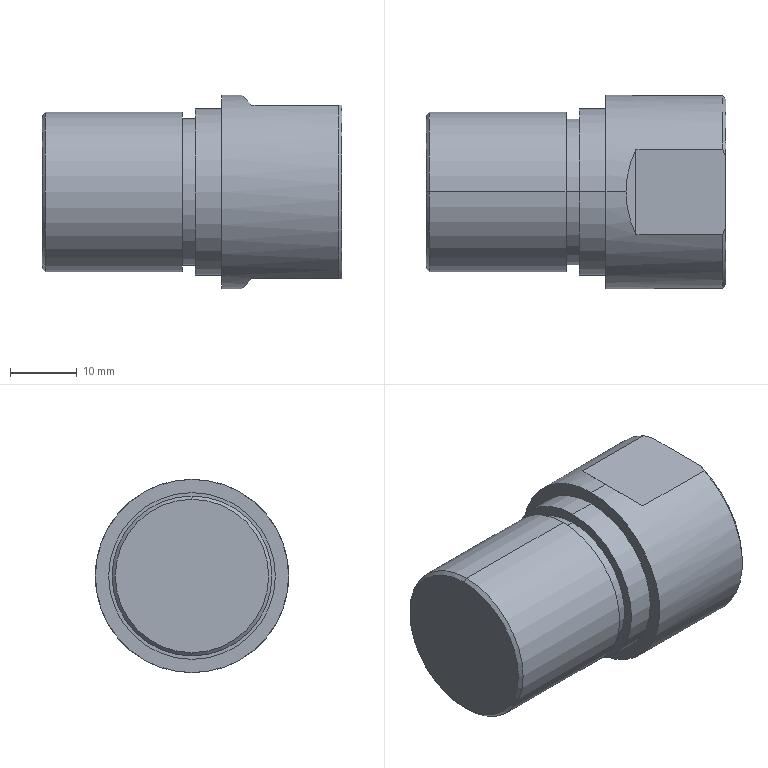Part | STEP file | 1 solid | 25 faces | box 45 x 29 x 29 mm | volume 22988 mm3 | cylinder 10 | plane 9 | cone 6 | commonest cylinder face diameters 6.8 x2 22 x2 24 x2 25 x2 29 x2
STEP:
#1=CARTESIAN_POINT('',(34.25,0.,3.4));
#2=VERTEX_POINT('',#1);
#3=CARTESIAN_POINT('',(34.25,0.,-3.4));
#4=VERTEX_POINT('',#3);
#5=CARTESIAN_POINT('',(34.25,0.,0.));
#6=DIRECTION('',(1.,0.,0.));
#7=DIRECTION('',(0.,0.,-1.));
#8=AXIS2_PLACEMENT_3D('',#5,#6,#7);
#9=CIRCLE('',#8,3.4);
#10=EDGE_CURVE('',#2,#4,#9,.T.);
#11=ORIENTED_EDGE('',*,*,#10,.F.);
#12=CARTESIAN_POINT('',(54.,0.,3.4));
#13=VERTEX_POINT('',#12);
#14=CARTESIAN_POINT('',(54.,0.,3.4));
#15=DIRECTION('',(1.,0.,0.));
#16=VECTOR('',#15,1000.);
#17=LINE('',#14,#16);
#18=EDGE_CURVE('',#2,#13,#17,.T.);
#19=ORIENTED_EDGE('',*,*,#18,.T.);
#20=CARTESIAN_POINT('',(54.,0.,-3.4));
#21=VERTEX_POINT('',#20);
#22=CARTESIAN_POINT('',(54.,0.,0.));
#23=DIRECTION('',(1.,0.,0.));
#24=DIRECTION('',(0.,0.,-1.));
#25=AXIS2_PLACEMENT_3D('',#22,#23,#24);
#26=CIRCLE('',#25,3.4);
#27=EDGE_CURVE('',#13,#21,#26,.T.);
#28=ORIENTED_EDGE('',*,*,#27,.T.);
#29=CARTESIAN_POINT('',(54.,0.,-3.4));
#30=DIRECTION('',(1.,0.,0.));
#31=VECTOR('',#30,1000.);
#32=LINE('',#29,#31);
#33=EDGE_CURVE('',#4,#21,#32,.T.);
#34=ORIENTED_EDGE('',*,*,#33,.F.);
#35=EDGE_LOOP('',(#11,#19,#28,#34));
#36=FACE_OUTER_BOUND('',#35,.T.);
#37=CARTESIAN_POINT('',(54.,0.,0.));
#38=DIRECTION('',(1.,0.,0.));
#39=DIRECTION('',(0.,0.,-1.));
#40=AXIS2_PLACEMENT_3D('',#37,#38,#39);
#41=CYLINDRICAL_SURFACE('',#40,3.4);
#42=ADVANCED_FACE('',(#36),#41,.F.);
#43=CARTESIAN_POINT('',(32.207,0.,0.));
#44=VERTEX_POINT('',#43);
#45=CARTESIAN_POINT('',(34.25,0.,-3.4));
#46=DIRECTION('',(0.515,0.,-0.8572));
#47=VECTOR('',#46,1000.);
#48=LINE('',#45,#47);
#49=EDGE_CURVE('',#44,#4,#48,.T.);
#50=ORIENTED_EDGE('',*,*,#49,.F.);
#51=CARTESIAN_POINT('',(34.25,0.,3.4));
#52=DIRECTION('',(0.515,0.,0.8572));
#53=VECTOR('',#52,1000.);
#54=LINE('',#51,#53);
#55=EDGE_CURVE('',#44,#2,#54,.T.);
#56=ORIENTED_EDGE('',*,*,#55,.T.);
#57=ORIENTED_EDGE('',*,*,#10,.T.);
#58=EDGE_LOOP('',(#50,#56,#57));
#59=FACE_OUTER_BOUND('',#58,.T.);
#60=CARTESIAN_POINT('',(34.25,0.,0.));
#61=DIRECTION('',(1.,0.,0.));
#62=DIRECTION('',(0.,0.,-1.));
#63=AXIS2_PLACEMENT_3D('',#60,#61,#62);
#64=CONICAL_SURFACE('',#63,3.4,1.03);
#65=ADVANCED_FACE('',(#59),#64,.F.);
#66=CARTESIAN_POINT('',(9.,0.,11.5));
#67=VERTEX_POINT('',#66);
#68=CARTESIAN_POINT('',(9.,0.,-11.5));
#69=VERTEX_POINT('',#68);
#70=CARTESIAN_POINT('',(9.,0.,0.));
#71=DIRECTION('',(-1.,0.,0.));
#72=DIRECTION('',(0.,0.,1.));
#73=AXIS2_PLACEMENT_3D('',#70,#71,#72);
#74=CIRCLE('',#73,11.5);
#75=EDGE_CURVE('',#67,#69,#74,.T.);
#76=ORIENTED_EDGE('',*,*,#75,.F.);
#77=CARTESIAN_POINT('',(9.5,0.,12.));
#78=VERTEX_POINT('',#77);
#79=CARTESIAN_POINT('',(9.,0.,11.5));
#80=DIRECTION('',(0.7071,0.,0.7071));
#81=VECTOR('',#80,1000.);
#82=LINE('',#79,#81);
#83=EDGE_CURVE('',#67,#78,#82,.T.);
#84=ORIENTED_EDGE('',*,*,#83,.T.);
#85=CARTESIAN_POINT('',(9.5,0.,-12.));
#86=VERTEX_POINT('',#85);
#87=CARTESIAN_POINT('',(9.5,0.,0.));
#88=DIRECTION('',(1.,0.,0.));
#89=DIRECTION('',(0.,0.,1.));
#90=AXIS2_PLACEMENT_3D('',#87,#88,#89);
#91=CIRCLE('',#90,12.);
#92=EDGE_CURVE('',#86,#78,#91,.T.);
#93=ORIENTED_EDGE('',*,*,#92,.F.);
#94=CARTESIAN_POINT('',(9.,0.,-11.5));
#95=DIRECTION('',(0.7071,0.,-0.7071));
#96=VECTOR('',#95,1000.);
#97=LINE('',#94,#96);
#98=EDGE_CURVE('',#69,#86,#97,.T.);
#99=ORIENTED_EDGE('',*,*,#98,.F.);
#100=EDGE_LOOP('',(#76,#84,#93,#99));
#101=FACE_OUTER_BOUND('',#100,.T.);
#102=CARTESIAN_POINT('',(9.,0.,0.));
#103=DIRECTION('',(1.,0.,0.));
#104=DIRECTION('',(0.,0.,-1.));
#105=AXIS2_PLACEMENT_3D('',#102,#103,#104);
#106=CONICAL_SURFACE('',#105,11.5,0.7854);
#107=ADVANCED_FACE('',(#101),#106,.T.);
#108=CARTESIAN_POINT('',(30.,0.,-12.));
#109=VERTEX_POINT('',#108);
#110=CARTESIAN_POINT('',(30.,0.,12.));
#111=VERTEX_POINT('',#110);
#112=CARTESIAN_POINT('',(30.,0.,0.));
#113=DIRECTION('',(1.,0.,0.));
#114=DIRECTION('',(0.,0.,1.));
#115=AXIS2_PLACEMENT_3D('',#112,#113,#114);
#116=CIRCLE('',#115,12.);
#117=EDGE_CURVE('',#109,#111,#116,.T.);
#118=ORIENTED_EDGE('',*,*,#117,.F.);
#119=CARTESIAN_POINT('',(36.,0.,-12.));
#120=DIRECTION('',(-1.,0.,0.));
#121=VECTOR('',#120,1000.);
#122=LINE('',#119,#121);
#123=EDGE_CURVE('',#109,#86,#122,.T.);
#124=ORIENTED_EDGE('',*,*,#123,.T.);
#125=ORIENTED_EDGE('',*,*,#92,.T.);
#126=CARTESIAN_POINT('',(36.,0.,12.));
#127=DIRECTION('',(-1.,0.,0.));
#128=VECTOR('',#127,1000.);
#129=LINE('',#126,#128);
#130=EDGE_CURVE('',#111,#78,#129,.T.);
#131=ORIENTED_EDGE('',*,*,#130,.F.);
#132=EDGE_LOOP('',(#118,#124,#125,#131));
#133=FACE_OUTER_BOUND('',#132,.T.);
#134=CARTESIAN_POINT('',(36.,0.,0.));
#135=DIRECTION('',(-1.,0.,0.));
#136=DIRECTION('',(0.,0.,1.));
#137=AXIS2_PLACEMENT_3D('',#134,#135,#136);
#138=CYLINDRICAL_SURFACE('',#137,12.);
#139=ADVANCED_FACE('',(#133),#138,.T.);
#140=CARTESIAN_POINT('',(30.,0.,11.));
#141=VERTEX_POINT('',#140);
#142=CARTESIAN_POINT('',(30.,0.,-11.));
#143=VERTEX_POINT('',#142);
#144=CARTESIAN_POINT('',(30.,0.,0.));
#145=DIRECTION('',(-1.,0.,0.));
#146=DIRECTION('',(0.,0.,1.));
#147=AXIS2_PLACEMENT_3D('',#144,#145,#146);
#148=CIRCLE('',#147,11.);
#149=EDGE_CURVE('',#141,#143,#148,.T.);
#150=ORIENTED_EDGE('',*,*,#149,.F.);
#151=CARTESIAN_POINT('',(32.,0.,11.));
#152=VERTEX_POINT('',#151);
#153=CARTESIAN_POINT('',(30.,0.,11.));
#154=DIRECTION('',(1.,0.,0.));
#155=VECTOR('',#154,1000.);
#156=LINE('',#153,#155);
#157=EDGE_CURVE('',#141,#152,#156,.T.);
#158=ORIENTED_EDGE('',*,*,#157,.T.);
#159=CARTESIAN_POINT('',(32.,0.,-11.));
#160=VERTEX_POINT('',#159);
#161=CARTESIAN_POINT('',(32.,0.,0.));
#162=DIRECTION('',(-1.,0.,0.));
#163=DIRECTION('',(0.,0.,1.));
#164=AXIS2_PLACEMENT_3D('',#161,#162,#163);
#165=CIRCLE('',#164,11.);
#166=EDGE_CURVE('',#152,#160,#165,.T.);
#167=ORIENTED_EDGE('',*,*,#166,.T.);
#168=CARTESIAN_POINT('',(30.,0.,-11.));
#169=DIRECTION('',(1.,0.,0.));
#170=VECTOR('',#169,1000.);
#171=LINE('',#168,#170);
#172=EDGE_CURVE('',#143,#160,#171,.T.);
#173=ORIENTED_EDGE('',*,*,#172,.F.);
#174=EDGE_LOOP('',(#150,#158,#167,#173));
#175=FACE_OUTER_BOUND('',#174,.T.);
#176=CARTESIAN_POINT('',(30.,0.,0.));
#177=DIRECTION('',(1.,0.,0.));
#178=DIRECTION('',(0.,0.,-1.));
#179=AXIS2_PLACEMENT_3D('',#176,#177,#178);
#180=CYLINDRICAL_SURFACE('',#179,11.);
#181=ADVANCED_FACE('',(#175),#180,.T.);
#182=CARTESIAN_POINT('',(32.,0.,12.5));
#183=VERTEX_POINT('',#182);
#184=CARTESIAN_POINT('',(32.,0.,-12.5));
#185=VERTEX_POINT('',#184);
#186=CARTESIAN_POINT('',(32.,0.,0.));
#187=DIRECTION('',(-1.,0.,0.));
#188=DIRECTION('',(0.,0.,1.));
#189=AXIS2_PLACEMENT_3D('',#186,#187,#188);
#190=CIRCLE('',#189,12.5);
#191=EDGE_CURVE('',#183,#185,#190,.T.);
#192=ORIENTED_EDGE('',*,*,#191,.F.);
#193=CARTESIAN_POINT('',(36.,0.,12.5));
#194=VERTEX_POINT('',#193);
#195=CARTESIAN_POINT('',(32.,0.,12.5));
#196=DIRECTION('',(1.,0.,0.));
#197=VECTOR('',#196,1000.);
#198=LINE('',#195,#197);
#199=EDGE_CURVE('',#183,#194,#198,.T.);
#200=ORIENTED_EDGE('',*,*,#199,.T.);
#201=CARTESIAN_POINT('',(36.,0.,-12.5));
#202=VERTEX_POINT('',#201);
#203=CARTESIAN_POINT('',(36.,0.,0.));
#204=DIRECTION('',(-1.,0.,0.));
#205=DIRECTION('',(0.,0.,1.));
#206=AXIS2_PLACEMENT_3D('',#203,#204,#205);
#207=CIRCLE('',#206,12.5);
#208=EDGE_CURVE('',#194,#202,#207,.T.);
#209=ORIENTED_EDGE('',*,*,#208,.T.);
#210=CARTESIAN_POINT('',(32.,0.,-12.5));
#211=DIRECTION('',(1.,0.,0.));
#212=VECTOR('',#211,1000.);
#213=LINE('',#210,#212);
#214=EDGE_CURVE('',#185,#202,#213,.T.);
#215=ORIENTED_EDGE('',*,*,#214,.F.);
#216=EDGE_LOOP('',(#192,#200,#209,#215));
#217=FACE_OUTER_BOUND('',#216,.T.);
#218=CARTESIAN_POINT('',(32.,0.,0.));
#219=DIRECTION('',(1.,0.,0.));
#220=DIRECTION('',(0.,0.,-1.));
#221=AXIS2_PLACEMENT_3D('',#218,#219,#220);
#222=CYLINDRICAL_SURFACE('',#221,12.5);
#223=ADVANCED_FACE('',(#217),#222,.T.);
#224=CARTESIAN_POINT('',(40.5,6.423,-13.));
#225=VERTEX_POINT('',#224);
#226=CARTESIAN_POINT('',(39.,0.,-14.5));
#227=VERTEX_POINT('',#226);
#228=CARTESIAN_POINT('',(40.5,6.423,-13.));
#229=CARTESIAN_POINT('',(39.509,4.417,-13.991));
#230=CARTESIAN_POINT('',(39.,2.238,-14.5));
#231=CARTESIAN_POINT('',(39.,0.,-14.5));
#232=(BOUNDED_CURVE()B_SPLINE_CURVE(3,(#228,#229,#230,#231),.UNSPECIFIED.,.F.,.F.)B_SPLINE_CURVE_WITH_KNOTS((4,4),(5.824,6.283),.UNSPECIFIED.)CURVE()GEOMETRIC_REPRESENTATION_ITEM()RATIONAL_B_SPLINE_CURVE((1.,0.9825,0.9825,1.))REPRESENTATION_ITEM(''));
#233=EDGE_CURVE('',#225,#227,#232,.T.);
#234=ORIENTED_EDGE('',*,*,#233,.T.);
#235=CARTESIAN_POINT('',(36.,0.,-14.5));
#236=VERTEX_POINT('',#235);
#237=CARTESIAN_POINT('',(94.001,0.,-14.5));
#238=DIRECTION('',(-1.,0.,0.));
#239=VECTOR('',#238,1000.);
#240=LINE('',#237,#239);
#241=EDGE_CURVE('',#227,#236,#240,.T.);
#242=ORIENTED_EDGE('',*,*,#241,.T.);
#243=CARTESIAN_POINT('',(36.,0.,14.5));
#244=VERTEX_POINT('',#243);
#245=CARTESIAN_POINT('',(36.,0.,0.));
#246=DIRECTION('',(-1.,0.,0.));
#247=DIRECTION('',(0.,0.,1.));
#248=AXIS2_PLACEMENT_3D('',#245,#246,#247);
#249=CIRCLE('',#248,14.5);
#250=EDGE_CURVE('',#244,#236,#249,.T.);
#251=ORIENTED_EDGE('',*,*,#250,.F.);
#252=CARTESIAN_POINT('',(39.,0.,14.5));
#253=VERTEX_POINT('',#252);
#254=CARTESIAN_POINT('',(94.001,0.,14.5));
#255=DIRECTION('',(-1.,0.,0.));
#256=VECTOR('',#255,1000.);
#257=LINE('',#254,#256);
#258=EDGE_CURVE('',#253,#244,#257,.T.);
#259=ORIENTED_EDGE('',*,*,#258,.F.);
#260=CARTESIAN_POINT('',(40.5,6.423,13.));
#261=VERTEX_POINT('',#260);
#262=CARTESIAN_POINT('',(39.,0.,14.5));
#263=CARTESIAN_POINT('',(39.,2.238,14.5));
#264=CARTESIAN_POINT('',(39.509,4.417,13.991));
#265=CARTESIAN_POINT('',(40.5,6.423,13.));
#266=(BOUNDED_CURVE()B_SPLINE_CURVE(3,(#262,#263,#264,#265),.UNSPECIFIED.,.F.,.F.)B_SPLINE_CURVE_WITH_KNOTS((4,4),(0.,0.4589),.UNSPECIFIED.)CURVE()GEOMETRIC_REPRESENTATION_ITEM()RATIONAL_B_SPLINE_CURVE((1.,0.9825,0.9825,1.))REPRESENTATION_ITEM(''));
#267=EDGE_CURVE('',#253,#261,#266,.T.);
#268=ORIENTED_EDGE('',*,*,#267,.T.);
#269=CARTESIAN_POINT('',(53.5,6.423,13.));
#270=VERTEX_POINT('',#269);
#271=CARTESIAN_POINT('',(94.001,6.423,13.));
#272=DIRECTION('',(-1.,0.,0.));
#273=VECTOR('',#272,1000.);
#274=LINE('',#271,#273);
#275=EDGE_CURVE('',#270,#261,#274,.T.);
#276=ORIENTED_EDGE('',*,*,#275,.F.);
#277=CARTESIAN_POINT('',(53.5,6.423,-13.));
#278=VERTEX_POINT('',#277);
#279=CARTESIAN_POINT('',(53.5,0.,0.));
#280=DIRECTION('',(-1.,0.,0.));
#281=DIRECTION('',(0.,0.,-1.));
#282=AXIS2_PLACEMENT_3D('',#279,#280,#281);
#283=CIRCLE('',#282,14.5);
#284=EDGE_CURVE('',#270,#278,#283,.T.);
#285=ORIENTED_EDGE('',*,*,#284,.T.);
#286=CARTESIAN_POINT('',(94.001,6.423,-13.));
#287=DIRECTION('',(1.,0.,0.));
#288=VECTOR('',#287,1000.);
#289=LINE('',#286,#288);
#290=EDGE_CURVE('',#225,#278,#289,.T.);
#291=ORIENTED_EDGE('',*,*,#290,.F.);
#292=EDGE_LOOP('',(#234,#242,#251,#259,#268,#276,#285,#291));
#293=FACE_OUTER_BOUND('',#292,.T.);
#294=CARTESIAN_POINT('',(94.001,0.,0.));
#295=DIRECTION('',(-1.,0.,0.));
#296=DIRECTION('',(0.,0.,1.));
#297=AXIS2_PLACEMENT_3D('',#294,#295,#296);
#298=CYLINDRICAL_SURFACE('',#297,14.5);
#299=ADVANCED_FACE('',(#293),#298,.T.);
#300=CARTESIAN_POINT('',(54.,5.196,13.));
#301=VERTEX_POINT('',#300);
#302=CARTESIAN_POINT('',(54.,-5.196,13.));
#303=VERTEX_POINT('',#302);
#304=CARTESIAN_POINT('',(54.,12.5,13.));
#305=DIRECTION('',(0.,-1.,0.));
#306=VECTOR('',#305,1000.);
#307=LINE('',#304,#306);
#308=EDGE_CURVE('',#301,#303,#307,.T.);
#309=ORIENTED_EDGE('',*,*,#308,.T.);
#310=CARTESIAN_POINT('',(54.,-5.196,-13.));
#311=VERTEX_POINT('',#310);
#312=CARTESIAN_POINT('',(54.,0.,0.));
#313=DIRECTION('',(1.,0.,0.));
#314=DIRECTION('',(0.,0.,-1.));
#315=AXIS2_PLACEMENT_3D('',#312,#313,#314);
#316=CIRCLE('',#315,14.);
#317=EDGE_CURVE('',#303,#311,#316,.T.);
#318=ORIENTED_EDGE('',*,*,#317,.T.);
#319=CARTESIAN_POINT('',(54.,5.196,-13.));
#320=VERTEX_POINT('',#319);
#321=CARTESIAN_POINT('',(54.,12.5,-13.));
#322=DIRECTION('',(0.,1.,0.));
#323=VECTOR('',#322,1000.);
#324=LINE('',#321,#323);
#325=EDGE_CURVE('',#311,#320,#324,.T.);
#326=ORIENTED_EDGE('',*,*,#325,.T.);
#327=CARTESIAN_POINT('',(54.,0.,0.));
#328=DIRECTION('',(1.,0.,0.));
#329=DIRECTION('',(0.,0.,-1.));
#330=AXIS2_PLACEMENT_3D('',#327,#328,#329);
#331=CIRCLE('',#330,14.);
#332=EDGE_CURVE('',#320,#301,#331,.T.);
#333=ORIENTED_EDGE('',*,*,#332,.T.);
#334=EDGE_LOOP('',(#309,#318,#326,#333));
#335=FACE_OUTER_BOUND('',#334,.T.);
#336=CARTESIAN_POINT('',(54.,0.,0.));
#337=DIRECTION('',(1.,0.,0.));
#338=DIRECTION('',(0.,0.,-1.));
#339=AXIS2_PLACEMENT_3D('',#336,#337,#338);
#340=CIRCLE('',#339,3.4);
#341=EDGE_CURVE('',#21,#13,#340,.T.);
#342=ORIENTED_EDGE('',*,*,#341,.F.);
#343=ORIENTED_EDGE('',*,*,#27,.F.);
#344=EDGE_LOOP('',(#342,#343));
#345=FACE_BOUND('',#344,.T.);
#346=CARTESIAN_POINT('',(54.,12.5,0.));
#347=DIRECTION('',(1.,0.,0.));
#348=DIRECTION('',(0.,1.,0.));
#349=AXIS2_PLACEMENT_3D('',#346,#347,#348);
#350=PLANE('',#349);
#351=ADVANCED_FACE('',(#335,#345),#350,.T.);
#352=ORIENTED_EDGE('',*,*,#250,.T.);
#353=CARTESIAN_POINT('',(36.,0.,0.));
#354=DIRECTION('',(-1.,0.,0.));
#355=DIRECTION('',(0.,0.,1.));
#356=AXIS2_PLACEMENT_3D('',#353,#354,#355);
#357=CIRCLE('',#356,14.5);
#358=EDGE_CURVE('',#236,#244,#357,.T.);
#359=ORIENTED_EDGE('',*,*,#358,.T.);
#360=EDGE_LOOP('',(#352,#359));
#361=FACE_OUTER_BOUND('',#360,.T.);
#362=CARTESIAN_POINT('',(36.,0.,0.));
#363=DIRECTION('',(-1.,0.,0.));
#364=DIRECTION('',(0.,0.,1.));
#365=AXIS2_PLACEMENT_3D('',#362,#363,#364);
#366=CIRCLE('',#365,12.5);
#367=EDGE_CURVE('',#202,#194,#366,.T.);
#368=ORIENTED_EDGE('',*,*,#367,.F.);
#369=ORIENTED_EDGE('',*,*,#208,.F.);
#370=EDGE_LOOP('',(#368,#369));
#371=FACE_BOUND('',#370,.T.);
#372=CARTESIAN_POINT('',(36.,0.,0.));
#373=DIRECTION('',(-1.,0.,0.));
#374=DIRECTION('',(0.,0.,1.));
#375=AXIS2_PLACEMENT_3D('',#372,#373,#374);
#376=PLANE('',#375);
#377=ADVANCED_FACE('',(#361,#371),#376,.T.);
#378=ORIENTED_EDGE('',*,*,#241,.F.);
#379=CARTESIAN_POINT('',(40.5,-6.423,-13.));
#380=VERTEX_POINT('',#379);
#381=CARTESIAN_POINT('',(39.,0.,-14.5));
#382=CARTESIAN_POINT('',(39.,-2.238,-14.5));
#383=CARTESIAN_POINT('',(39.509,-4.417,-13.991));
#384=CARTESIAN_POINT('',(40.5,-6.423,-13.));
#385=(BOUNDED_CURVE()B_SPLINE_CURVE(3,(#381,#382,#383,#384),.UNSPECIFIED.,.F.,.F.)B_SPLINE_CURVE_WITH_KNOTS((4,4),(0.,0.4589),.UNSPECIFIED.)CURVE()GEOMETRIC_REPRESENTATION_ITEM()RATIONAL_B_SPLINE_CURVE((1.,0.9825,0.9825,1.))REPRESENTATION_ITEM(''));
#386=EDGE_CURVE('',#227,#380,#385,.T.);
#387=ORIENTED_EDGE('',*,*,#386,.T.);
#388=CARTESIAN_POINT('',(53.5,-6.423,-13.));
#389=VERTEX_POINT('',#388);
#390=CARTESIAN_POINT('',(94.001,-6.423,-13.));
#391=DIRECTION('',(-1.,0.,0.));
#392=VECTOR('',#391,1000.);
#393=LINE('',#390,#392);
#394=EDGE_CURVE('',#389,#380,#393,.T.);
#395=ORIENTED_EDGE('',*,*,#394,.F.);
#396=CARTESIAN_POINT('',(53.5,-6.423,13.));
#397=VERTEX_POINT('',#396);
#398=CARTESIAN_POINT('',(53.5,0.,0.));
#399=DIRECTION('',(-1.,0.,0.));
#400=DIRECTION('',(0.,0.,-1.));
#401=AXIS2_PLACEMENT_3D('',#398,#399,#400);
#402=CIRCLE('',#401,14.5);
#403=EDGE_CURVE('',#389,#397,#402,.T.);
#404=ORIENTED_EDGE('',*,*,#403,.T.);
#405=CARTESIAN_POINT('',(40.5,-6.423,13.));
#406=VERTEX_POINT('',#405);
#407=CARTESIAN_POINT('',(94.001,-6.423,13.));
#408=DIRECTION('',(1.,0.,0.));
#409=VECTOR('',#408,1000.);
#410=LINE('',#407,#409);
#411=EDGE_CURVE('',#406,#397,#410,.T.);
#412=ORIENTED_EDGE('',*,*,#411,.F.);
#413=CARTESIAN_POINT('',(40.5,-6.423,13.));
#414=CARTESIAN_POINT('',(39.509,-4.417,13.991));
#415=CARTESIAN_POINT('',(39.,-2.238,14.5));
#416=CARTESIAN_POINT('',(39.,0.,14.5));
#417=(BOUNDED_CURVE()B_SPLINE_CURVE(3,(#413,#414,#415,#416),.UNSPECIFIED.,.F.,.F.)B_SPLINE_CURVE_WITH_KNOTS((4,4),(5.824,6.283),.UNSPECIFIED.)CURVE()GEOMETRIC_REPRESENTATION_ITEM()RATIONAL_B_SPLINE_CURVE((1.,0.9825,0.9825,1.))REPRESENTATION_ITEM(''));
#418=EDGE_CURVE('',#406,#253,#417,.T.);
#419=ORIENTED_EDGE('',*,*,#418,.T.);
#420=ORIENTED_EDGE('',*,*,#258,.T.);
#421=ORIENTED_EDGE('',*,*,#358,.F.);
#422=EDGE_LOOP('',(#378,#387,#395,#404,#412,#419,#420,#421));
#423=FACE_OUTER_BOUND('',#422,.T.);
#424=CARTESIAN_POINT('',(94.001,0.,0.));
#425=DIRECTION('',(-1.,0.,0.));
#426=DIRECTION('',(0.,0.,1.));
#427=AXIS2_PLACEMENT_3D('',#424,#425,#426);
#428=CYLINDRICAL_SURFACE('',#427,14.5);
#429=ADVANCED_FACE('',(#423),#428,.T.);
#430=CARTESIAN_POINT('',(40.5,7.483,-13.));
#431=DIRECTION('',(0.,-1.,0.));
#432=VECTOR('',#431,1000.);
#433=LINE('',#430,#432);
#434=EDGE_CURVE('',#225,#380,#433,.T.);
#435=ORIENTED_EDGE('',*,*,#434,.T.);
#436=ORIENTED_EDGE('',*,*,#386,.F.);
#437=ORIENTED_EDGE('',*,*,#233,.F.);
#438=EDGE_LOOP('',(#435,#436,#437));
#439=FACE_OUTER_BOUND('',#438,.T.);
#440=CARTESIAN_POINT('',(40.5,7.483,-13.));
#441=DIRECTION('',(0.7071,0.,-0.7071));
#442=DIRECTION('',(0.,-1.,0.));
#443=AXIS2_PLACEMENT_3D('',#440,#441,#442);
#444=PLANE('',#443);
#445=ADVANCED_FACE('',(#439),#444,.T.);
#446=CARTESIAN_POINT('',(40.5,-7.483,13.));
#447=DIRECTION('',(0.,1.,0.));
#448=VECTOR('',#447,1000.);
#449=LINE('',#446,#448);
#450=EDGE_CURVE('',#406,#261,#449,.T.);
#451=ORIENTED_EDGE('',*,*,#450,.T.);
#452=ORIENTED_EDGE('',*,*,#267,.F.);
#453=ORIENTED_EDGE('',*,*,#418,.F.);
#454=EDGE_LOOP('',(#451,#452,#453));
#455=FACE_OUTER_BOUND('',#454,.T.);
#456=CARTESIAN_POINT('',(40.5,-7.483,13.));
#457=DIRECTION('',(0.7071,0.,0.7071));
#458=DIRECTION('',(0.,-1.,0.));
#459=AXIS2_PLACEMENT_3D('',#456,#457,#458);
#460=PLANE('',#459);
#461=ADVANCED_FACE('',(#455),#460,.T.);
#462=ORIENTED_EDGE('',*,*,#411,.T.);
#463=CARTESIAN_POINT('',(53.5,-6.423,13.));
#464=CARTESIAN_POINT('',(53.679,-6.019,13.));
#465=CARTESIAN_POINT('',(53.846,-5.61,13.));
#466=CARTESIAN_POINT('',(54.,-5.196,13.));
#467=B_SPLINE_CURVE_WITH_KNOTS('',3,(#463,#464,#465,#466),.UNSPECIFIED.,.F.,.F.,(4,4),(0.,0.001324),.UNSPECIFIED.);
#468=EDGE_CURVE('',#397,#303,#467,.T.);
#469=ORIENTED_EDGE('',*,*,#468,.T.);
#470=ORIENTED_EDGE('',*,*,#308,.F.);
#471=CARTESIAN_POINT('',(54.,5.196,13.));
#472=CARTESIAN_POINT('',(53.846,5.61,13.));
#473=CARTESIAN_POINT('',(53.679,6.019,13.));
#474=CARTESIAN_POINT('',(53.5,6.423,13.));
#475=B_SPLINE_CURVE_WITH_KNOTS('',3,(#471,#472,#473,#474),.UNSPECIFIED.,.F.,.F.,(4,4),(0.,0.001324),.UNSPECIFIED.);
#476=EDGE_CURVE('',#301,#270,#475,.T.);
#477=ORIENTED_EDGE('',*,*,#476,.T.);
#478=ORIENTED_EDGE('',*,*,#275,.T.);
#479=ORIENTED_EDGE('',*,*,#450,.F.);
#480=EDGE_LOOP('',(#462,#469,#470,#477,#478,#479));
#481=FACE_OUTER_BOUND('',#480,.T.);
#482=CARTESIAN_POINT('',(54.,0.,13.));
#483=DIRECTION('',(0.,0.,-1.));
#484=DIRECTION('',(0.,-1.,0.));
#485=AXIS2_PLACEMENT_3D('',#482,#483,#484);
#486=PLANE('',#485);
#487=ADVANCED_FACE('',(#481),#486,.F.);
#488=ORIENTED_EDGE('',*,*,#325,.F.);
#489=CARTESIAN_POINT('',(54.,-5.196,-13.));
#490=CARTESIAN_POINT('',(53.846,-5.61,-13.));
#491=CARTESIAN_POINT('',(53.679,-6.019,-13.));
#492=CARTESIAN_POINT('',(53.5,-6.423,-13.));
#493=B_SPLINE_CURVE_WITH_KNOTS('',3,(#489,#490,#491,#492),.UNSPECIFIED.,.F.,.F.,(4,4),(0.,0.001324),.UNSPECIFIED.);
#494=EDGE_CURVE('',#311,#389,#493,.T.);
#495=ORIENTED_EDGE('',*,*,#494,.T.);
#496=ORIENTED_EDGE('',*,*,#394,.T.);
#497=ORIENTED_EDGE('',*,*,#434,.F.);
#498=ORIENTED_EDGE('',*,*,#290,.T.);
#499=CARTESIAN_POINT('',(53.5,6.423,-13.));
#500=CARTESIAN_POINT('',(53.679,6.019,-13.));
#501=CARTESIAN_POINT('',(53.846,5.61,-13.));
#502=CARTESIAN_POINT('',(54.,5.196,-13.));
#503=B_SPLINE_CURVE_WITH_KNOTS('',3,(#499,#500,#501,#502),.UNSPECIFIED.,.F.,.F.,(4,4),(0.,0.001324),.UNSPECIFIED.);
#504=EDGE_CURVE('',#278,#320,#503,.T.);
#505=ORIENTED_EDGE('',*,*,#504,.T.);
#506=EDGE_LOOP('',(#488,#495,#496,#497,#498,#505));
#507=FACE_OUTER_BOUND('',#506,.T.);
#508=CARTESIAN_POINT('',(54.,0.,-13.));
#509=DIRECTION('',(0.,0.,1.));
#510=DIRECTION('',(1.,0.,0.));
#511=AXIS2_PLACEMENT_3D('',#508,#509,#510);
#512=PLANE('',#511);
#513=ADVANCED_FACE('',(#507),#512,.F.);
#514=ORIENTED_EDGE('',*,*,#199,.F.);
#515=CARTESIAN_POINT('',(32.,0.,0.));
#516=DIRECTION('',(-1.,0.,0.));
#517=DIRECTION('',(0.,0.,1.));
#518=AXIS2_PLACEMENT_3D('',#515,#516,#517);
#519=CIRCLE('',#518,12.5);
#520=EDGE_CURVE('',#185,#183,#519,.T.);
#521=ORIENTED_EDGE('',*,*,#520,.F.);
#522=ORIENTED_EDGE('',*,*,#214,.T.);
#523=ORIENTED_EDGE('',*,*,#367,.T.);
#524=EDGE_LOOP('',(#514,#521,#522,#523));
#525=FACE_OUTER_BOUND('',#524,.T.);
#526=CARTESIAN_POINT('',(32.,0.,0.));
#527=DIRECTION('',(1.,0.,0.));
#528=DIRECTION('',(0.,0.,-1.));
#529=AXIS2_PLACEMENT_3D('',#526,#527,#528);
#530=CYLINDRICAL_SURFACE('',#529,12.5);
#531=ADVANCED_FACE('',(#525),#530,.T.);
#532=ORIENTED_EDGE('',*,*,#520,.T.);
#533=ORIENTED_EDGE('',*,*,#191,.T.);
#534=EDGE_LOOP('',(#532,#533));
#535=FACE_OUTER_BOUND('',#534,.T.);
#536=CARTESIAN_POINT('',(32.,0.,0.));
#537=DIRECTION('',(-1.,0.,0.));
#538=DIRECTION('',(0.,0.,1.));
#539=AXIS2_PLACEMENT_3D('',#536,#537,#538);
#540=CIRCLE('',#539,11.);
#541=EDGE_CURVE('',#160,#152,#540,.T.);
#542=ORIENTED_EDGE('',*,*,#541,.F.);
#543=ORIENTED_EDGE('',*,*,#166,.F.);
#544=EDGE_LOOP('',(#542,#543));
#545=FACE_BOUND('',#544,.T.);
#546=CARTESIAN_POINT('',(32.,0.,0.));
#547=DIRECTION('',(-1.,0.,0.));
#548=DIRECTION('',(0.,0.,1.));
#549=AXIS2_PLACEMENT_3D('',#546,#547,#548);
#550=PLANE('',#549);
#551=ADVANCED_FACE('',(#535,#545),#550,.T.);
#552=CARTESIAN_POINT('',(30.,0.,0.));
#553=DIRECTION('',(1.,0.,0.));
#554=DIRECTION('',(0.,0.,1.));
#555=AXIS2_PLACEMENT_3D('',#552,#553,#554);
#556=CIRCLE('',#555,12.);
#557=EDGE_CURVE('',#111,#109,#556,.T.);
#558=ORIENTED_EDGE('',*,*,#557,.T.);
#559=ORIENTED_EDGE('',*,*,#117,.T.);
#560=EDGE_LOOP('',(#558,#559));
#561=FACE_OUTER_BOUND('',#560,.T.);
#562=CARTESIAN_POINT('',(30.,0.,0.));
#563=DIRECTION('',(-1.,0.,0.));
#564=DIRECTION('',(0.,0.,1.));
#565=AXIS2_PLACEMENT_3D('',#562,#563,#564);
#566=CIRCLE('',#565,11.);
#567=EDGE_CURVE('',#143,#141,#566,.T.);
#568=ORIENTED_EDGE('',*,*,#567,.T.);
#569=ORIENTED_EDGE('',*,*,#149,.T.);
#570=EDGE_LOOP('',(#568,#569));
#571=FACE_BOUND('',#570,.T.);
#572=CARTESIAN_POINT('',(30.,0.,0.));
#573=DIRECTION('',(-1.,0.,0.));
#574=DIRECTION('',(0.,0.,1.));
#575=AXIS2_PLACEMENT_3D('',#572,#573,#574);
#576=PLANE('',#575);
#577=ADVANCED_FACE('',(#561,#571),#576,.F.);
#578=ORIENTED_EDGE('',*,*,#157,.F.);
#579=ORIENTED_EDGE('',*,*,#567,.F.);
#580=ORIENTED_EDGE('',*,*,#172,.T.);
#581=ORIENTED_EDGE('',*,*,#541,.T.);
#582=EDGE_LOOP('',(#578,#579,#580,#581));
#583=FACE_OUTER_BOUND('',#582,.T.);
#584=CARTESIAN_POINT('',(30.,0.,0.));
#585=DIRECTION('',(1.,0.,0.));
#586=DIRECTION('',(0.,0.,-1.));
#587=AXIS2_PLACEMENT_3D('',#584,#585,#586);
#588=CYLINDRICAL_SURFACE('',#587,11.);
#589=ADVANCED_FACE('',(#583),#588,.T.);
#590=ORIENTED_EDGE('',*,*,#123,.F.);
#591=ORIENTED_EDGE('',*,*,#557,.F.);
#592=ORIENTED_EDGE('',*,*,#130,.T.);
#593=CARTESIAN_POINT('',(9.5,0.,0.));
#594=DIRECTION('',(1.,0.,0.));
#595=DIRECTION('',(0.,0.,1.));
#596=AXIS2_PLACEMENT_3D('',#593,#594,#595);
#597=CIRCLE('',#596,12.);
#598=EDGE_CURVE('',#78,#86,#597,.T.);
#599=ORIENTED_EDGE('',*,*,#598,.T.);
#600=EDGE_LOOP('',(#590,#591,#592,#599));
#601=FACE_OUTER_BOUND('',#600,.T.);
#602=CARTESIAN_POINT('',(36.,0.,0.));
#603=DIRECTION('',(-1.,0.,0.));
#604=DIRECTION('',(0.,0.,1.));
#605=AXIS2_PLACEMENT_3D('',#602,#603,#604);
#606=CYLINDRICAL_SURFACE('',#605,12.);
#607=ADVANCED_FACE('',(#601),#606,.T.);
#608=CARTESIAN_POINT('',(9.,0.,0.));
#609=DIRECTION('',(-1.,0.,0.));
#610=DIRECTION('',(0.,0.,1.));
#611=AXIS2_PLACEMENT_3D('',#608,#609,#610);
#612=CIRCLE('',#611,11.5);
#613=EDGE_CURVE('',#69,#67,#612,.T.);
#614=ORIENTED_EDGE('',*,*,#613,.T.);
#615=ORIENTED_EDGE('',*,*,#75,.T.);
#616=EDGE_LOOP('',(#614,#615));
#617=FACE_OUTER_BOUND('',#616,.T.);
#618=CARTESIAN_POINT('',(9.,0.,0.));
#619=DIRECTION('',(-1.,0.,0.));
#620=DIRECTION('',(0.,0.,1.));
#621=AXIS2_PLACEMENT_3D('',#618,#619,#620);
#622=PLANE('',#621);
#623=ADVANCED_FACE('',(#617),#622,.T.);
#624=ORIENTED_EDGE('',*,*,#83,.F.);
#625=ORIENTED_EDGE('',*,*,#613,.F.);
#626=ORIENTED_EDGE('',*,*,#98,.T.);
#627=ORIENTED_EDGE('',*,*,#598,.F.);
#628=EDGE_LOOP('',(#624,#625,#626,#627));
#629=FACE_OUTER_BOUND('',#628,.T.);
#630=CARTESIAN_POINT('',(9.,0.,0.));
#631=DIRECTION('',(1.,0.,0.));
#632=DIRECTION('',(0.,0.,-1.));
#633=AXIS2_PLACEMENT_3D('',#630,#631,#632);
#634=CONICAL_SURFACE('',#633,11.5,0.7854);
#635=ADVANCED_FACE('',(#629),#634,.T.);
#636=ORIENTED_EDGE('',*,*,#55,.F.);
#637=ORIENTED_EDGE('',*,*,#49,.T.);
#638=CARTESIAN_POINT('',(34.25,0.,0.));
#639=DIRECTION('',(1.,0.,0.));
#640=DIRECTION('',(0.,0.,-1.));
#641=AXIS2_PLACEMENT_3D('',#638,#639,#640);
#642=CIRCLE('',#641,3.4);
#643=EDGE_CURVE('',#4,#2,#642,.T.);
#644=ORIENTED_EDGE('',*,*,#643,.T.);
#645=EDGE_LOOP('',(#636,#637,#644));
#646=FACE_OUTER_BOUND('',#645,.T.);
#647=CARTESIAN_POINT('',(34.25,0.,0.));
#648=DIRECTION('',(1.,0.,0.));
#649=DIRECTION('',(0.,0.,-1.));
#650=AXIS2_PLACEMENT_3D('',#647,#648,#649);
#651=CONICAL_SURFACE('',#650,3.4,1.03);
#652=ADVANCED_FACE('',(#646),#651,.F.);
#653=ORIENTED_EDGE('',*,*,#18,.F.);
#654=ORIENTED_EDGE('',*,*,#643,.F.);
#655=ORIENTED_EDGE('',*,*,#33,.T.);
#656=ORIENTED_EDGE('',*,*,#341,.T.);
#657=EDGE_LOOP('',(#653,#654,#655,#656));
#658=FACE_OUTER_BOUND('',#657,.T.);
#659=CARTESIAN_POINT('',(54.,0.,0.));
#660=DIRECTION('',(1.,0.,0.));
#661=DIRECTION('',(0.,0.,-1.));
#662=AXIS2_PLACEMENT_3D('',#659,#660,#661);
#663=CYLINDRICAL_SURFACE('',#662,3.4);
#664=ADVANCED_FACE('',(#658),#663,.F.);
#665=ORIENTED_EDGE('',*,*,#494,.F.);
#666=ORIENTED_EDGE('',*,*,#317,.F.);
#667=ORIENTED_EDGE('',*,*,#468,.F.);
#668=ORIENTED_EDGE('',*,*,#403,.F.);
#669=EDGE_LOOP('',(#665,#666,#667,#668));
#670=FACE_OUTER_BOUND('',#669,.T.);
#671=CARTESIAN_POINT('',(53.5,0.,0.));
#672=DIRECTION('',(-1.,0.,0.));
#673=DIRECTION('',(0.,0.,1.));
#674=AXIS2_PLACEMENT_3D('',#671,#672,#673);
#675=CONICAL_SURFACE('',#674,14.5,0.7854);
#676=ADVANCED_FACE('',(#670),#675,.T.);
#677=ORIENTED_EDGE('',*,*,#476,.F.);
#678=ORIENTED_EDGE('',*,*,#332,.F.);
#679=ORIENTED_EDGE('',*,*,#504,.F.);
#680=ORIENTED_EDGE('',*,*,#284,.F.);
#681=EDGE_LOOP('',(#677,#678,#679,#680));
#682=FACE_OUTER_BOUND('',#681,.T.);
#683=CARTESIAN_POINT('',(53.5,0.,0.));
#684=DIRECTION('',(-1.,0.,0.));
#685=DIRECTION('',(0.,0.,1.));
#686=AXIS2_PLACEMENT_3D('',#683,#684,#685);
#687=CONICAL_SURFACE('',#686,14.5,0.7854);
#688=ADVANCED_FACE('',(#682),#687,.T.);
#689=CLOSED_SHELL('',(#42,#65,#107,#139,#181,#223,#299,#351,#377,#429,#445,#461,#487,#513,#531,#551,#577,#589,#607,#623,#635,#652,#664,#676,#688));
#690=MANIFOLD_SOLID_BREP('',#689);
#691=CARTESIAN_POINT('',(0.,0.,0.));
#692=DIRECTION('',(0.,0.,1.));
#693=DIRECTION('',(1.,0.,0.));
#694=AXIS2_PLACEMENT_3D('',#691,#692,#693);
#695=(LENGTH_UNIT()NAMED_UNIT(*)SI_UNIT(.MILLI.,.METRE.));
#696=UNCERTAINTY_MEASURE_WITH_UNIT(LENGTH_MEASURE(0.00001),#695,'','');
#697=(NAMED_UNIT(*)PLANE_ANGLE_UNIT()SI_UNIT($,.RADIAN.));
#698=(NAMED_UNIT(*)SI_UNIT($,.STERADIAN.)SOLID_ANGLE_UNIT());
#699=(GEOMETRIC_REPRESENTATION_CONTEXT(3)GLOBAL_UNCERTAINTY_ASSIGNED_CONTEXT((#696))GLOBAL_UNIT_ASSIGNED_CONTEXT((#695,#697,#698))REPRESENTATION_CONTEXT('',''));
#700=ADVANCED_BREP_SHAPE_REPRESENTATION('',(#690,#694),#699);